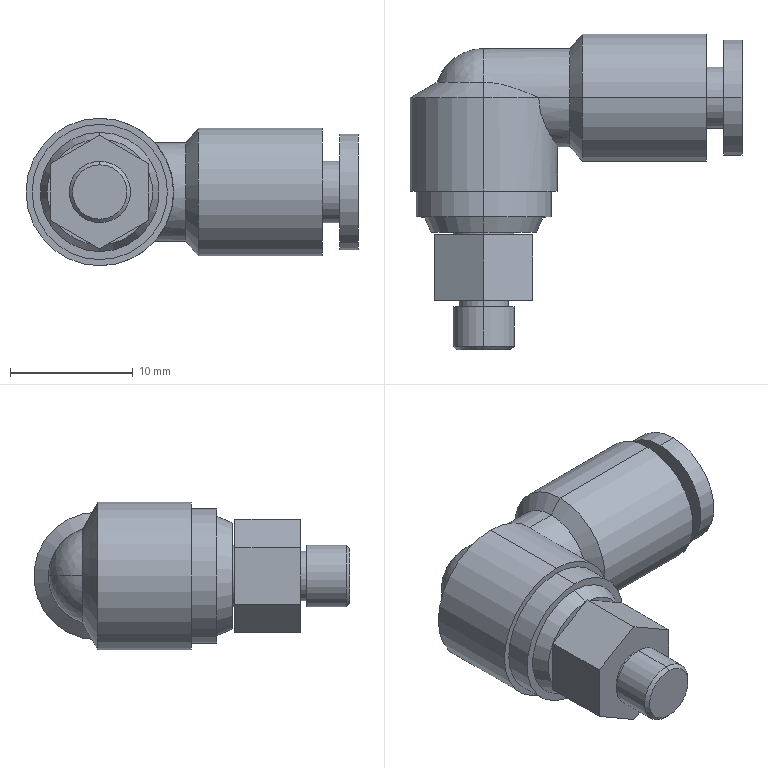Part | STEP file | KSL04-M5 | 1 solid | 48 faces | box 27 x 25.7 x 12 mm | volume 2672 mm3 | cylinder 20 | plane 17 | cone 9 | spline 2 | commonest cylinder face diameters 5 x6 4 x2 4.02 x2 8 x2 9.4 x2 10.4 x2